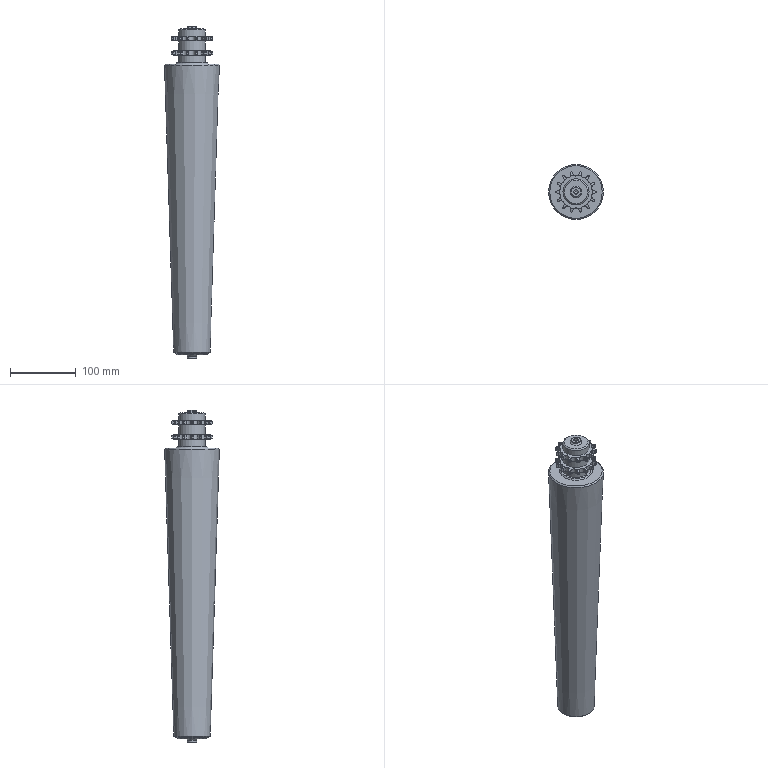Part | STEP file | 08b1-14 | 1 solid | 308 faces | box 83.871 x 83.871 x 506 mm | volume 1796791 mm3 | cylinder 173 | plane 68 | torus 56 | cone 8 | spline 3 | commonest cylinder face diameters 14.27 x56 22.211 x56 8.595 x28 63.262 x28 40 x3 14 x2